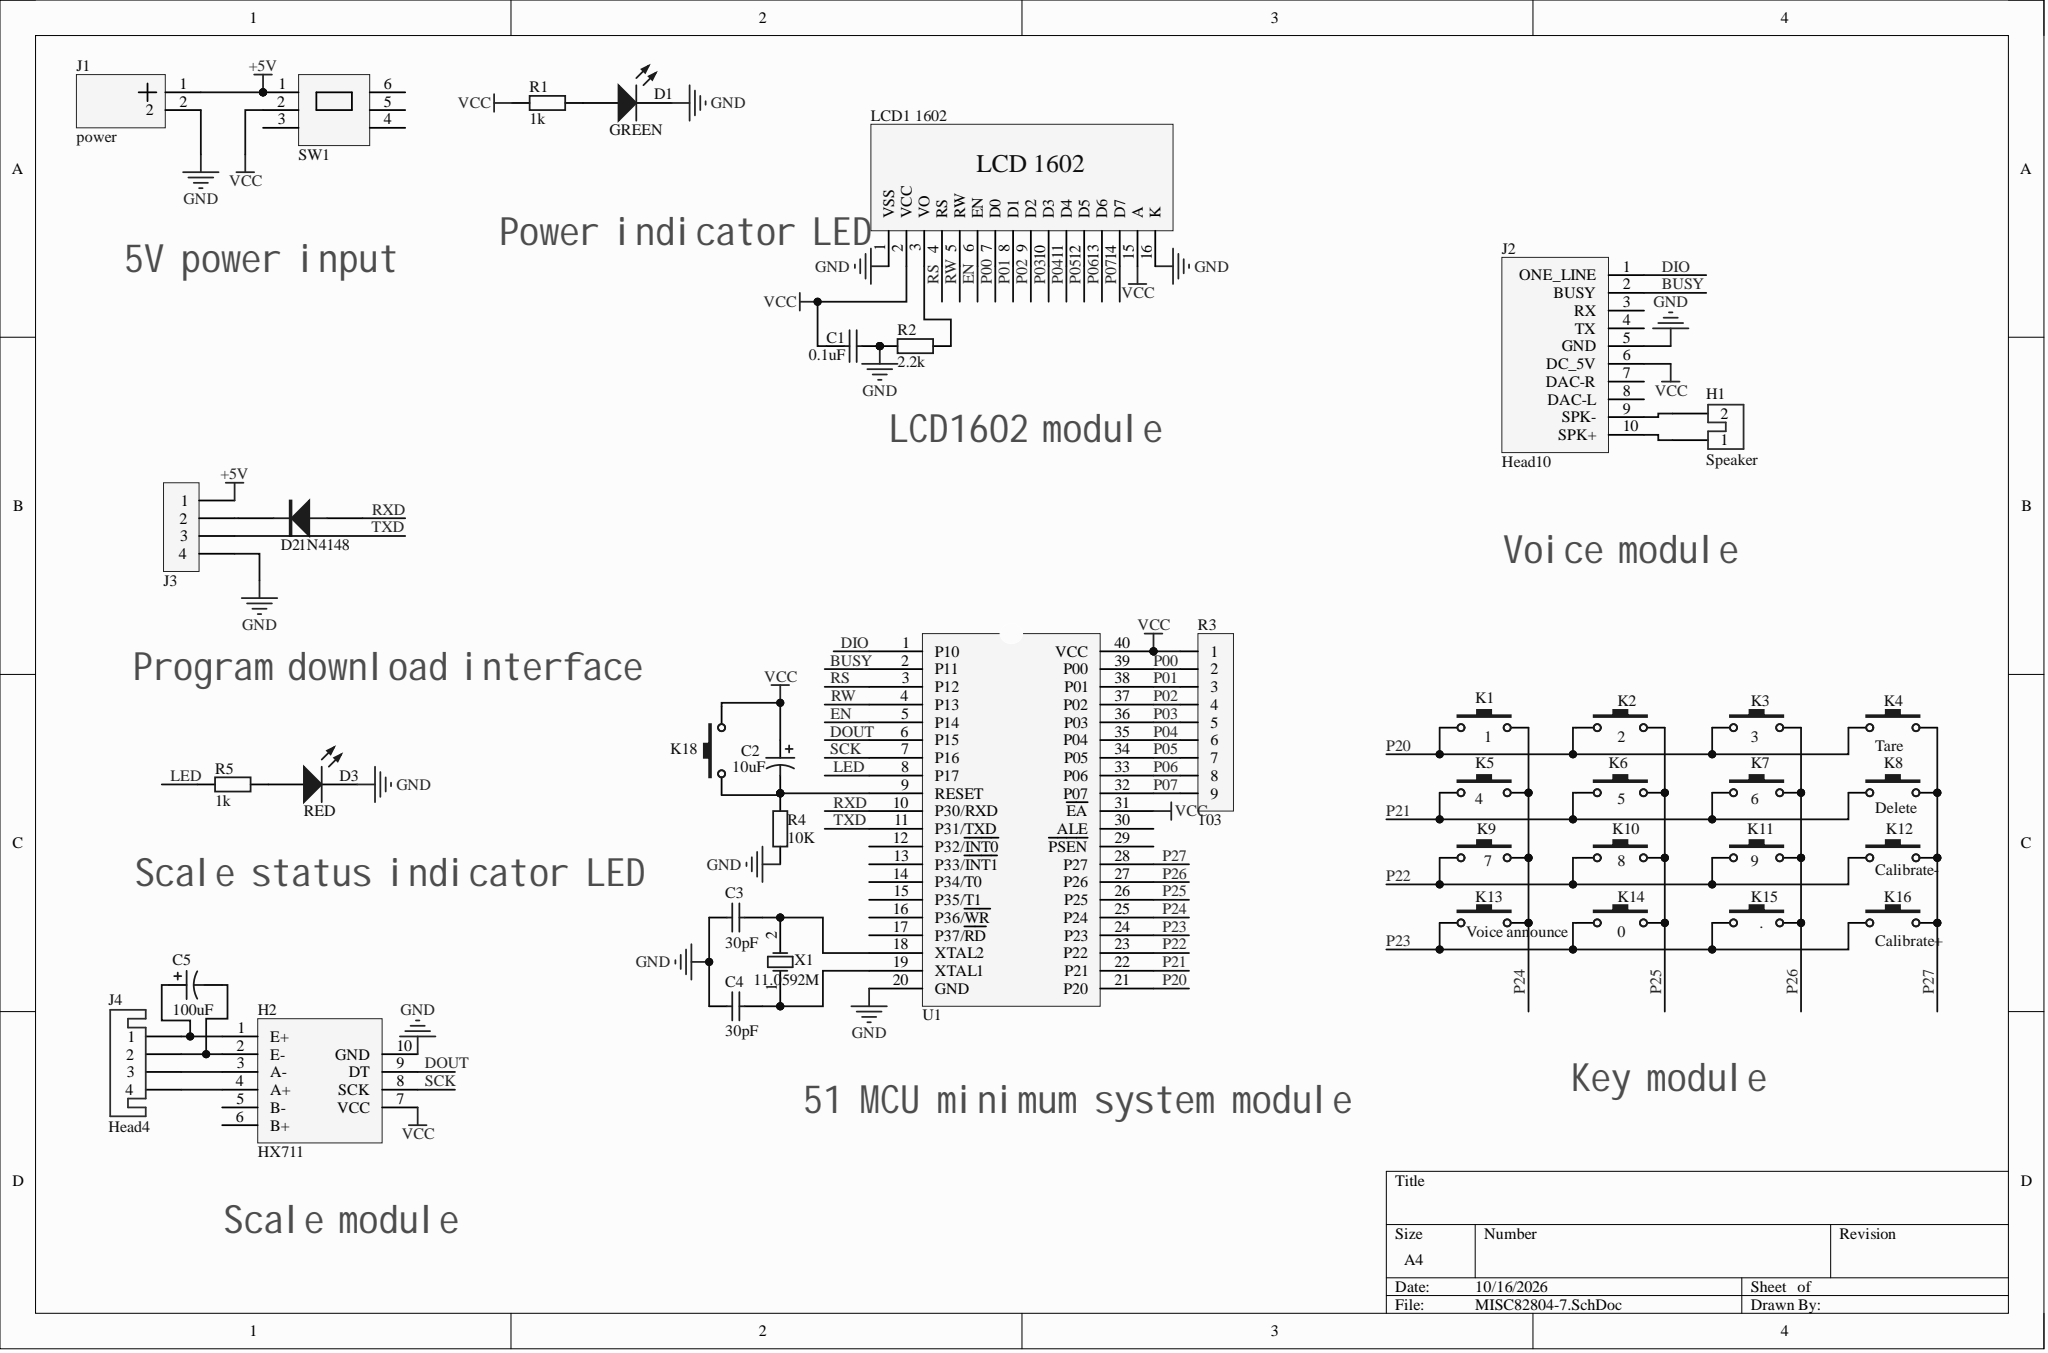Circuit board | Altium Designer | 40 parts | 42 nets
Bill of materials:
Comment,Description,Designator,Footprint,LibRef,Quantity
"0.1uF","Capacitor","C1","CAP","CAP","1"
"10uF","","C2","CAP_1","CAP_2","1"
"30pF","","C3, C4","CAP","CAP","2"
"100uF","","C5","CAP_2","CAP_2","1"
"GREEN","","D1","LED_3MM_GREEN_1C-2A - duplicate","LED","1"
"1N4148","","D2","1N4148","1N4148","1"
"RED","","D3","LED_3MM_RED_1C-2A","LED","1"
"Speaker","","H1","609-2p-vr130","Head2","1"
"HX711","","H2","hx711","HX7111","1"
"power","","J1","DC3.5 - me","DC5.5","1"
"Head10","","J2","10PIN语音模块","Head10","1"
"SENSOR","","J3","4PIN","CON4","1"
"Head4","","J4","609-4p-vr130","Head4","1"
"1","","K1","SW2","KEY","1"
"2","","K2","SW2","KEY","1"
"3","","K3","SW2","KEY","1"
"Tare","","K4","SW2","KEY","1"
"4","","K5","SW2","KEY","1"
"5","","K6","SW2","KEY","1"
"6","","K7","SW2","KEY","1"
"Delete","","K8","SW2","KEY","1"
"7","","K9","SW2","KEY","1"
"8","","K10","SW2","KEY","1"
"9","","K11","SW2","KEY","1"
"Calibrate-","","K12","SW2","KEY","1"
"Voice announce","","K13","SW2","KEY","1"
"0","","K14","SW2","KEY","1"
".","","K15","SW2","KEY","1"
"Calibrate+","","K16","SW2","KEY","1"
"KEY","","K18","SW2","KEY","1"
"1602","","LCD1","1602","1602","1"
"1k","","R1, R5","电阻-RM7.5-C","Res","2"
"2.2k","","R2","电阻-RM7.5-C","Res","1"
"103","","R3","PAIRES","Header9","1"
"10K","","R4","电阻-RM7.5-C","Res","1"
"SWT","","SW1","KEY-6","SWT","1"
"STC89C52","","U1","C51","STC89C52","1"
"11.059M","","X1","12M","XTAL","1"
Netlist (Protel format):
[
C1
CAP
0.1uF



]
[
C2
CAP_1
10uF



]
[
C3
CAP
30pF



]
[
C4
CAP
30pF



]
[
C5
CAP_2
100uF



]
[
D1
LED_3MM_GREEN_1C-2A - duplicate
GREEN



]
[
D2
1N4148
1N4148



]
[
D3
LED_3MM_RED_1C-2A
RED



]
[
H1
609-2p-vr130
Speaker



]
[
H2
hx711
HX711



]
[
J1
DC3.5 - me
power



]
[
J2
10PIN语音模块
Head10



]
[
J3
4PIN
SENSOR



]
[
J4
609-4p-vr130
Head4



]
[
K1
SW2
1



]
[
K2
SW2
2



]
[
K3
SW2
3



]
[
K4
SW2
Tare



]
[
K5
SW2
4



]
[
K6
SW2
5



]
[
K7
SW2
6



]
[
K8
SW2
Delete



]
[
K9
SW2
7



]
[
K10
SW2
8



]
[
K11
SW2
9



]
[
K12
SW2
Calibrate-



]
[
K13
SW2
Voice announce



]
[
K14
SW2
0



]
[
K15
SW2
.



]
[
K16
SW2
Calibrate+



]
[
K18
SW2
KEY



]
[
LCD1
1602
1602



]
[
R1
电阻-RM7.5-C
1k



]
[
R2
电阻-RM7.5-C
2.2k



]
[
R3
PAIRES
103



]
[
R4
电阻-RM7.5-C
10K



]
[
R5
电阻-RM7.5-C
1k



]
[
SW1
KEY-6
SWT



]
[
U1
C51
STC89C52



]
[
X1
12M
11.0592M



]
(
VCC
C1-2
C2-1
H2-7
J2-6
K18-2
LCD1-2
LCD1-15
R1-1
R3-1
SW1-2
U1-31
U1-40
)
(
TXD
J3-3
U1-11
)
(
SCK
H2-8
U1-7
)
(
RXD
D2-1
U1-10
)
(
RW
LCD1-5
U1-4
)
(
RS
LCD1-4
U1-3
)
(
P27
K4-2
K8-2
K12-2
K16-2
U1-28
)
(
P26
K3-2
K7-2
K11-2
K15-2
U1-27
)
(
P25
K2-2
K6-2
K10-2
K14-2
U1-26
)
(
P24
K1-2
K5-2
K9-2
K13-2
U1-25
)
(
P23
K13-1
K14-1
K15-1
K16-1
U1-24
)
(
P22
K9-1
K10-1
K11-1
K12-1
U1-23
)
(
P21
K5-1
K6-1
K7-1
K8-1
U1-22
)
(
P20
K1-1
K2-1
K3-1
K4-1
U1-21
)
(
P07
LCD1-14
R3-9
U1-32
)
(
P06
LCD1-13
R3-8
U1-33
)
(
P05
LCD1-12
R3-7
U1-34
)
(
P04
LCD1-11
R3-6
U1-35
)
(
P03
LCD1-10
R3-5
U1-36
)
(
P02
LCD1-9
R3-4
U1-37
)
(
P01
LCD1-8
R3-3
U1-38
)
(
P00
LCD1-7
R3-2
U1-39
)
(
NetLCD1_3
LCD1-3
R2-1
)
(
NetH2_4
H2-4
J4-4
)
(
NetH2_3
H2-3
J4-3
)
(
NetH1_2
H1-2
J2-9
)
(
NetH1_1
H1-1
J2-10
)
(
NetD3_1
D3-1
R5-2
)
(
NetD2_2
D2-2
J3-2
)
(
NetD1_1
D1-1
R1-2
)
(
NetC5_2
C5-2
H2-2
J4-2
)
(
NetC5_1
C5-1
H2-1
J4-1
)
(
NetC4_2
C4-2
U1-19
X1-1
)
(
NetC3_2
C3-2
U1-18
X1-2
)
(
NetC2_2
C2-2
K18-1
R4-2
U1-9
)
(
LED
R5-1
U1-8
)
(
GND
C1-1
C3-1
C4-1
D1-2
D3-2
H2-10
J1-2
J2-5
J3-4
LCD1-1
LCD1-16
R2-2
R4-1
U1-20
)
(
EN
LCD1-6
U1-5
)
(
DOUT
H2-9
U1-6
)
(
DIO
J2-1
U1-1
)
(
BUSY
J2-2
U1-2
)
(
+5V
J1-1
J3-1
SW1-1
)